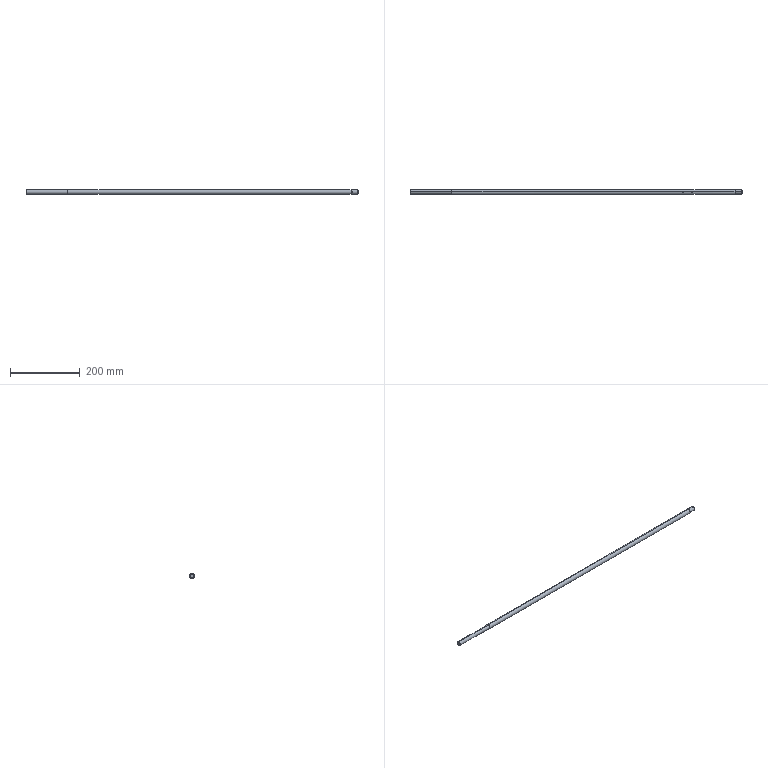Part | STEP file | adjusting screw rod 5_SUS304 | 1 solid | 20 faces | box 950 x 14 x 14 mm | volume 140280 mm3 | cylinder 12 | cone 4 | plane 4 | commonest cylinder face diameters 3 x4 12 x4 2 x2 14 x2